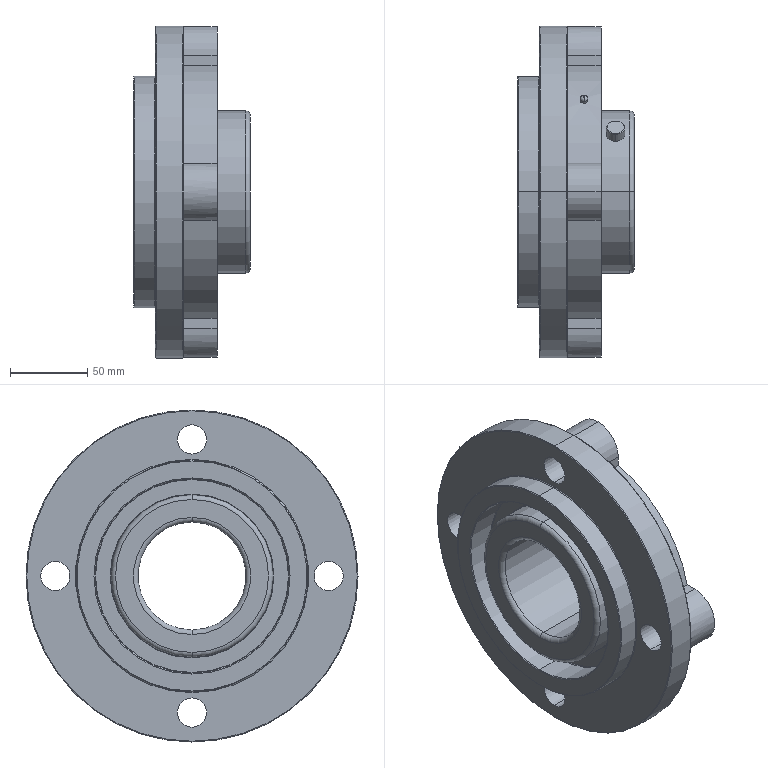Part | SolidWorks | features Revolution 3, ICE 2, Fillet 1 | 1 solid | 90 faces | box 75.4 x 215 x 215 mm | volume 1165108 mm3 | cylinder 37 | torus 26 | plane 23 | cone 4 | commonest cylinder face diameters 18.918 x8 37.082 x5 105 x4 167.459 x4 5 x2 12 x2